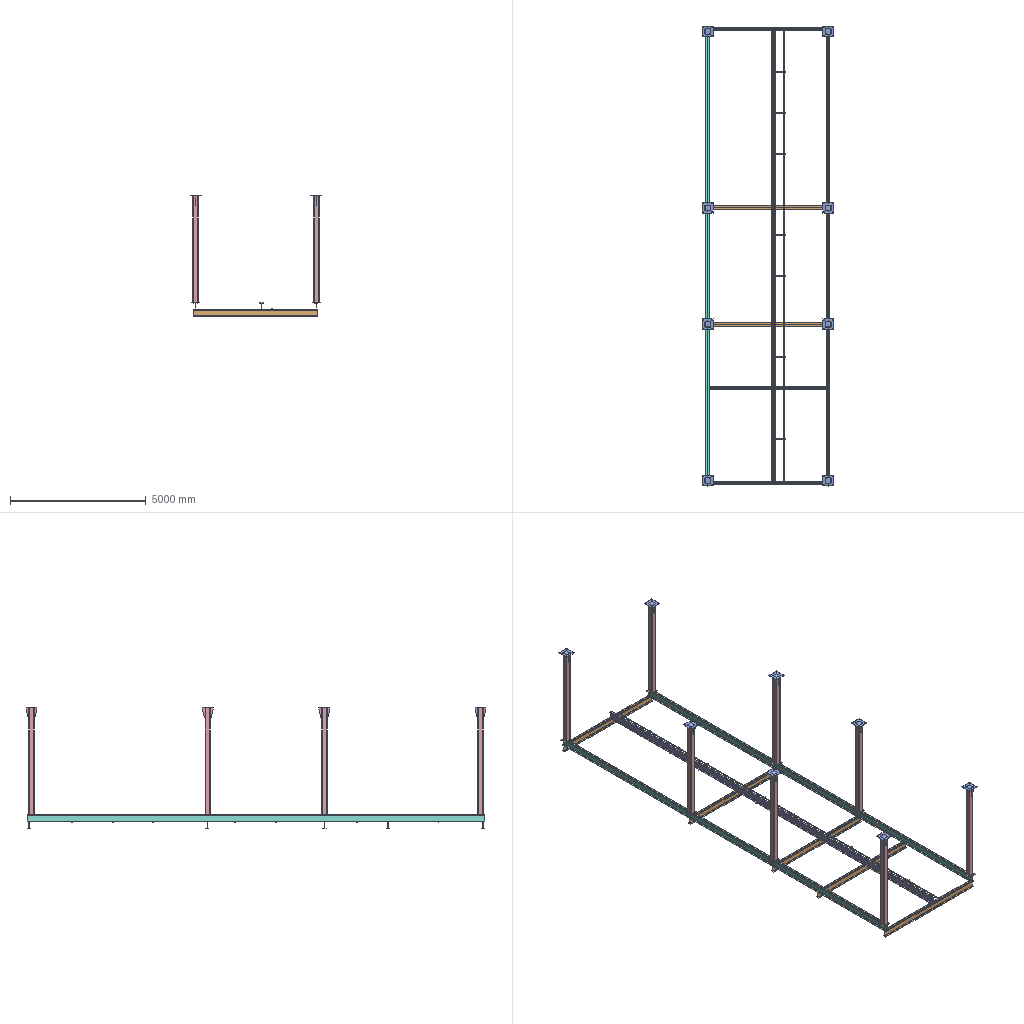Assembly | SolidWorks | 10 different items | 64 placed | box 4845 x 16940 x 4450 mm
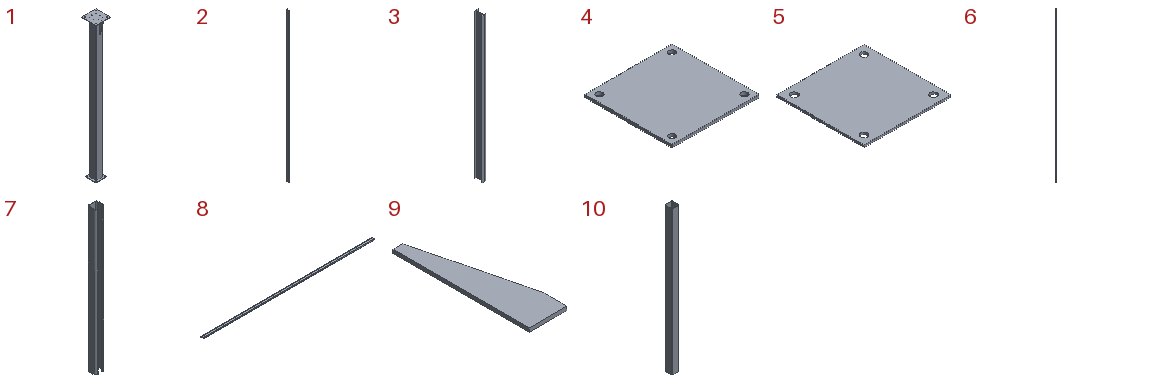Parts list (item | name | quantity | parent item | size | volume | features):
1 | (subassembly) | x8 | - | 400 x 400 x 3950 mm | 17687255 mm3 | -
2 | - | x2 | - | 125 x 250 x 16840 mm | 62256437 mm3 | features Extrusion 1
3 | - | x5 | - | 125 x 250 x 4570 mm | 16895007 mm3 | features Extrusion 1
4 | - | x8 | in 1 | 300 x 300 x 10 mm | 884795 mm3 | features Extrusion 1
5 | - | x8 | in 1 | 400 x 400 x 10 mm | 1567830 mm3 | features Extrusion 1
6 | - | x1 | - | 32 x 30 x 16840 mm | 2880981 mm3 | features Extrusion 1
7 | - | x7 | - | 32 x 30 x 500 mm | 85540 mm3 | features Extrusion 1
8 | - | x1 | - | 16840 x 250 x 118 mm | 87084540 mm3 | features Fillet 2, Extrusion 1
9 | - | x16 | in 1 | 100 x 360 x 10 mm | 249000 mm3 | features Extrusion 1
10 | - | x8 | in 1 | 200 x 200 x 3930 mm | 14736630 mm3 | features Extrusion 1
Mates (type | each side: item.copy, entity, surface, feature):
In the top assembly
Coincident | 4.1 face plane Boss-Extrude1 | 4.2 face plane Boss-Extrude1 | 2 times
Coincident | 4.1 face plane Boss-Extrude1 | 4.3 face plane Boss-Extrude1 | 2 times
Coincident | 4.1 face plane Boss-Extrude1 | 4.4 face plane Boss-Extrude1
Coincident | 4.1 face plane Boss-Extrude1 | 4.5 face plane Boss-Extrude1
Coincident | 4.1 face plane Boss-Extrude1 | 4.6 face plane Boss-Extrude1
Coincident | 4.1 face plane Boss-Extrude1 | 4.7 face plane Boss-Extrude1
Coincident | 4.1 face plane Boss-Extrude1 | 4.8 face plane Boss-Extrude1
Coincident | 4.3 face plane Boss-Extrude1 | 4.8 face plane Boss-Extrude1
Coincident | 4.8 face plane Boss-Extrude1 | 4.7 face plane Boss-Extrude1
Coincident | 4.2 face plane Boss-Extrude1 | 4.4 face plane Boss-Extrude1
Coincident | 4.2 face plane Boss-Extrude1 | 4.5 face plane Boss-Extrude1
Coincident | 4.2 face plane Boss-Extrude1 | 4.6 face plane Boss-Extrude1
Coincident | 4.6 face plane Boss-Extrude1 | 4.7 face plane Boss-Extrude1
Coincident | 4.5 face plane Boss-Extrude1 | 4.8 face plane Boss-Extrude1
Coincident | 4.3 face plane Boss-Extrude1 | 4.4 face plane Boss-Extrude1
DistanceDim | 4.1 face plane Boss-Extrude1 | 4.3 face plane Boss-Extrude1
DistanceDim | 4.3 face plane Boss-Extrude1 | 4.7 face plane Boss-Extrude1
Coincident | 4.1 face plane Boss-Extrude1 | 2.1 face plane Boss-Extrude1 | 2 times
Coincident | 2.1 face plane Boss-Extrude1 | 2.2 face plane Boss-Extrude1 | 2 times
DistanceDim | 4.2 face plane Boss-Extrude1 | 2.2 face plane Boss-Extrude1
Coincident | 3.1 face plane Boss-Extrude1 | 3.2 face plane Boss-Extrude1 | 2 times
Coincident | 3.1 face plane Boss-Extrude1 | 3.3 face plane Boss-Extrude1 | 2 times
Coincident | 3.1 face plane Boss-Extrude1 | 3.4 face plane Boss-Extrude1 | 2 times
Coincident | 3.1 face plane Boss-Extrude1 | 3.5 face plane Boss-Extrude1 | 2 times
Coincident | 2.2 face plane Boss-Extrude1 | 3.1 face plane Boss-Extrude1
Coincident | 2.1 face plane Boss-Extrude1 | 3.1 face plane Boss-Extrude1 | 2 times
Coincident | 2.1 face plane Boss-Extrude1 | 3.4 face plane Boss-Extrude1
DistanceDim | 10.1 face plane Boss-Extrude1 | 10.2 face plane Boss-Extrude1
Coincident | 3.1 face plane Boss-Extrude1 | 8.1 face plane Base | 2 times
DistanceDim | 8.1 face plane Base | 10.2 face plane Boss-Extrude1
DistanceDim | 4.8 face plane Boss-Extrude1 | 4.1 face plane Boss-Extrude1
Coincident | 2.2 face plane Boss-Extrude1 | 3.5 face plane Boss-Extrude1
Coincident | 3.1 face plane Boss-Extrude1 | 6.1 face plane Boss-Extrude1 | 2 times
DistanceDim | 6.1 face plane Boss-Extrude1 | 8.1 face plane Base
Coincident | 8.1 face plane Base | 7.1 face plane Boss-Extrude1
DistanceDim | 7.1 face plane Boss-Extrude1 | 6.1 face plane Boss-Extrude1
DistanceDim | 7.1 face plane Boss-Extrude1 | 3.1 face plane Boss-Extrude1
In subassembly 1
Coincident | 10.3 face plane Boss-Extrude1 | 5.1 face plane Boss-Extrude1
DistanceDim | 10.3 face plane Boss-Extrude1 | 5.1 face plane Boss-Extrude1 | 2 times
Coincident | 10.3 face plane Boss-Extrude1 | 4.9 face plane Boss-Extrude1
DistanceDim | 4.9 face plane Boss-Extrude1 | 10.3 face plane Boss-Extrude1 | 2 times
Coincident | 5.1 face plane Boss-Extrude1 | 9.1 face plane Boss-Extrude1
Coincident | 10.3 face plane Boss-Extrude1 | 9.1 face plane Boss-Extrude1
DistanceDim | 9.1 face plane Boss-Extrude1 | 5.1 face plane Boss-Extrude1
Coincident | 5.1 face plane Boss-Extrude1 | 9.2 face plane Boss-Extrude1
Coincident | 9.1 face plane Boss-Extrude1 | 9.2 face plane Boss-Extrude1
Coincident | 10.3 face plane Boss-Extrude1 | 9.2 face plane Boss-Extrude1